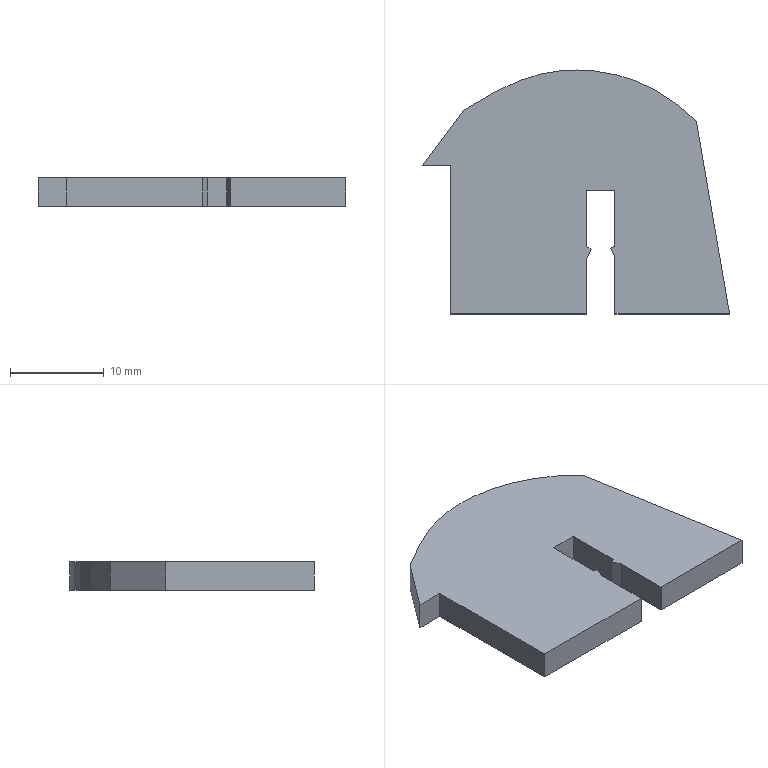Part | SolidWorks | features BaseBody 1 | 1 solid | 19 faces | box 32.694 x 25.985 x 3 mm | volume 1909 mm3 | plane 15 | spline 4
STEP:
#1=CARTESIAN_POINT('',(11.999,19.781,-1.5));
#2=VERTEX_POINT('',#1);
#3=CARTESIAN_POINT('',(15.525,-0.7188,-1.5));
#4=VERTEX_POINT('',#3);
#5=CARTESIAN_POINT('',(11.999,19.781,-1.5));
#6=CARTESIAN_POINT('',(12.867,14.683,-1.5));
#7=CARTESIAN_POINT('',(15.525,-0.7188,-1.5));
#8=B_SPLINE_CURVE_WITH_KNOTS('',2,(#5,#6,#7),.UNSPECIFIED.,.F.,.F.,(3,3),(0.3846,0.4615),.UNSPECIFIED.);
#9=EDGE_CURVE('',#2,#4,#8,.T.);
#10=ORIENTED_EDGE('',*,*,#9,.T.);
#11=CARTESIAN_POINT('',(3.329,-0.7188,-1.5));
#12=VERTEX_POINT('',#11);
#13=CARTESIAN_POINT('',(0.,-0.7188,-1.5));
#14=DIRECTION('',(-1.,0.,0.));
#15=VECTOR('',#14,1000.);
#16=LINE('',#13,#15);
#17=EDGE_CURVE('',#4,#12,#16,.T.);
#18=ORIENTED_EDGE('',*,*,#17,.T.);
#19=CARTESIAN_POINT('',(3.329,5.255,-1.5));
#20=VERTEX_POINT('',#19);
#21=CARTESIAN_POINT('',(3.329,0.,-1.5));
#22=DIRECTION('',(0.,-1.,0.));
#23=VECTOR('',#22,1000.);
#24=LINE('',#21,#23);
#25=EDGE_CURVE('',#20,#12,#24,.T.);
#26=ORIENTED_EDGE('',*,*,#25,.F.);
#27=CARTESIAN_POINT('',(2.879,6.296,-1.5));
#28=VERTEX_POINT('',#27);
#29=CARTESIAN_POINT('',(4.72,2.043,-1.5));
#30=DIRECTION('',(0.3973,-0.9177,0.));
#31=VECTOR('',#30,1000.);
#32=LINE('',#29,#31);
#33=EDGE_CURVE('',#28,#20,#32,.T.);
#34=ORIENTED_EDGE('',*,*,#33,.F.);
#35=CARTESIAN_POINT('',(3.329,6.492,-1.5));
#36=VERTEX_POINT('',#35);
#37=CARTESIAN_POINT('',(-1.842,4.249,-1.5));
#38=DIRECTION('',(-0.9175,-0.3978,0.));
#39=VECTOR('',#38,1000.);
#40=LINE('',#37,#39);
#41=EDGE_CURVE('',#36,#28,#40,.T.);
#42=ORIENTED_EDGE('',*,*,#41,.F.);
#43=CARTESIAN_POINT('',(3.329,12.466,-1.5));
#44=VERTEX_POINT('',#43);
#45=CARTESIAN_POINT('',(3.329,0.,-1.5));
#46=DIRECTION('',(0.,-1.,0.));
#47=VECTOR('',#46,1000.);
#48=LINE('',#45,#47);
#49=EDGE_CURVE('',#44,#36,#48,.T.);
#50=ORIENTED_EDGE('',*,*,#49,.F.);
#51=CARTESIAN_POINT('',(0.3317,12.466,-1.5));
#52=VERTEX_POINT('',#51);
#53=CARTESIAN_POINT('',(0.,12.466,-1.5));
#54=DIRECTION('',(1.,0.,0.));
#55=VECTOR('',#54,1000.);
#56=LINE('',#53,#55);
#57=EDGE_CURVE('',#52,#44,#56,.T.);
#58=ORIENTED_EDGE('',*,*,#57,.F.);
#59=CARTESIAN_POINT('',(0.3337,6.459,-1.5));
#60=VERTEX_POINT('',#59);
#61=CARTESIAN_POINT('',(0.3358,0.0001118,-1.5));
#62=DIRECTION('',(-0.000333,1.,0.));
#63=VECTOR('',#62,1000.);
#64=LINE('',#61,#63);
#65=EDGE_CURVE('',#60,#52,#64,.T.);
#66=ORIENTED_EDGE('',*,*,#65,.F.);
#67=CARTESIAN_POINT('',(0.7826,6.196,-1.5));
#68=VERTEX_POINT('',#67);
#69=CARTESIAN_POINT('',(2.904,4.951,-1.5));
#70=DIRECTION('',(-0.8626,0.5059,0.));
#71=VECTOR('',#70,1000.);
#72=LINE('',#69,#71);
#73=EDGE_CURVE('',#68,#60,#72,.T.);
#74=ORIENTED_EDGE('',*,*,#73,.F.);
#75=CARTESIAN_POINT('',(0.3337,5.236,-1.5));
#76=VERTEX_POINT('',#75);
#77=CARTESIAN_POINT('',(-1.736,0.8121,-1.5));
#78=DIRECTION('',(0.4237,0.9058,0.));
#79=VECTOR('',#78,1000.);
#80=LINE('',#77,#79);
#81=EDGE_CURVE('',#76,#68,#80,.T.);
#82=ORIENTED_EDGE('',*,*,#81,.F.);
#83=CARTESIAN_POINT('',(0.3337,-0.7188,-1.5));
#84=VERTEX_POINT('',#83);
#85=CARTESIAN_POINT('',(0.3337,0.,-1.5));
#86=DIRECTION('',(0.,1.,0.));
#87=VECTOR('',#86,1000.);
#88=LINE('',#85,#87);
#89=EDGE_CURVE('',#84,#76,#88,.T.);
#90=ORIENTED_EDGE('',*,*,#89,.F.);
#91=CARTESIAN_POINT('',(-14.173,-0.7188,-1.5));
#92=VERTEX_POINT('',#91);
#93=CARTESIAN_POINT('',(0.,-0.7188,-1.5));
#94=DIRECTION('',(-1.,0.,0.));
#95=VECTOR('',#94,1000.);
#96=LINE('',#93,#95);
#97=EDGE_CURVE('',#84,#92,#96,.T.);
#98=ORIENTED_EDGE('',*,*,#97,.T.);
#99=CARTESIAN_POINT('',(-14.173,15.089,-1.5));
#100=VERTEX_POINT('',#99);
#101=CARTESIAN_POINT('',(-14.173,0.,-1.5));
#102=DIRECTION('',(0.,1.,0.));
#103=VECTOR('',#102,1000.);
#104=LINE('',#101,#103);
#105=EDGE_CURVE('',#92,#100,#104,.T.);
#106=ORIENTED_EDGE('',*,*,#105,.T.);
#107=CARTESIAN_POINT('',(-17.169,15.089,-1.5));
#108=VERTEX_POINT('',#107);
#109=CARTESIAN_POINT('',(0.,15.089,-1.5));
#110=DIRECTION('',(-1.,0.,0.));
#111=VECTOR('',#110,1000.);
#112=LINE('',#109,#111);
#113=EDGE_CURVE('',#100,#108,#112,.T.);
#114=ORIENTED_EDGE('',*,*,#113,.T.);
#115=CARTESIAN_POINT('',(-12.796,20.955,-1.5));
#116=VERTEX_POINT('',#115);
#117=CARTESIAN_POINT('',(-17.169,15.089,-1.5));
#118=CARTESIAN_POINT('',(-15.712,17.045,-1.5));
#119=CARTESIAN_POINT('',(-14.255,19.001,-1.5));
#120=CARTESIAN_POINT('',(-12.796,20.955,-1.5));
#121=B_SPLINE_CURVE_WITH_KNOTS('',3,(#117,#118,#119,#120),.UNSPECIFIED.,.F.,.F.,(4,4),(0.1538,0.2308),.UNSPECIFIED.);
#122=EDGE_CURVE('',#108,#116,#121,.T.);
#123=ORIENTED_EDGE('',*,*,#122,.T.);
#124=CARTESIAN_POINT('',(1.186,25.157,-1.5));
#125=VERTEX_POINT('',#124);
#126=CARTESIAN_POINT('',(-12.796,20.955,-1.5));
#127=CARTESIAN_POINT('',(-8.856,23.384,-1.5));
#128=CARTESIAN_POINT('',(-4.918,25.815,-1.5));
#129=CARTESIAN_POINT('',(1.186,25.157,-1.5));
#130=B_SPLINE_CURVE_WITH_KNOTS('',3,(#126,#127,#128,#129),.UNSPECIFIED.,.F.,.F.,(4,4),(0.2308,0.3077),.UNSPECIFIED.);
#131=EDGE_CURVE('',#116,#125,#130,.T.);
#132=ORIENTED_EDGE('',*,*,#131,.T.);
#133=CARTESIAN_POINT('',(1.186,25.157,-1.5));
#134=CARTESIAN_POINT('',(5.549,24.686,-1.5));
#135=CARTESIAN_POINT('',(9.134,22.646,-1.5));
#136=CARTESIAN_POINT('',(11.999,19.781,-1.5));
#137=B_SPLINE_CURVE_WITH_KNOTS('',3,(#133,#134,#135,#136),.UNSPECIFIED.,.F.,.F.,(4,4),(0.3077,0.3846),.UNSPECIFIED.);
#138=EDGE_CURVE('',#125,#2,#137,.T.);
#139=ORIENTED_EDGE('',*,*,#138,.T.);
#140=EDGE_LOOP('',(#10,#18,#26,#34,#42,#50,#58,#66,#74,#82,#90,#98,#106,#114,#123,#132,#139));
#141=FACE_OUTER_BOUND('',#140,.T.);
#142=CARTESIAN_POINT('',(0.,0.,-1.5));
#143=DIRECTION('',(0.,0.,1.));
#144=DIRECTION('',(1.,0.,0.));
#145=AXIS2_PLACEMENT_3D('',#142,#143,#144);
#146=PLANE('',#145);
#147=ADVANCED_FACE('',(#141),#146,.F.);
#148=CARTESIAN_POINT('',(11.999,19.781,1.5));
#149=VERTEX_POINT('',#148);
#150=CARTESIAN_POINT('',(15.525,-0.7188,1.5));
#151=VERTEX_POINT('',#150);
#152=CARTESIAN_POINT('',(11.999,19.781,1.5));
#153=CARTESIAN_POINT('',(12.867,14.683,1.5));
#154=CARTESIAN_POINT('',(15.525,-0.7188,1.5));
#155=B_SPLINE_CURVE_WITH_KNOTS('',2,(#152,#153,#154),.UNSPECIFIED.,.F.,.F.,(3,3),(0.3846,0.4615),.UNSPECIFIED.);
#156=EDGE_CURVE('',#149,#151,#155,.T.);
#157=ORIENTED_EDGE('',*,*,#156,.F.);
#158=CARTESIAN_POINT('',(1.186,25.157,1.5));
#159=VERTEX_POINT('',#158);
#160=CARTESIAN_POINT('',(1.186,25.157,1.5));
#161=CARTESIAN_POINT('',(5.549,24.686,1.5));
#162=CARTESIAN_POINT('',(9.134,22.646,1.5));
#163=CARTESIAN_POINT('',(11.999,19.781,1.5));
#164=B_SPLINE_CURVE_WITH_KNOTS('',3,(#160,#161,#162,#163),.UNSPECIFIED.,.F.,.F.,(4,4),(0.3077,0.3846),.UNSPECIFIED.);
#165=EDGE_CURVE('',#159,#149,#164,.T.);
#166=ORIENTED_EDGE('',*,*,#165,.F.);
#167=CARTESIAN_POINT('',(-12.796,20.955,1.5));
#168=VERTEX_POINT('',#167);
#169=CARTESIAN_POINT('',(-12.796,20.955,1.5));
#170=CARTESIAN_POINT('',(-8.856,23.384,1.5));
#171=CARTESIAN_POINT('',(-4.918,25.815,1.5));
#172=CARTESIAN_POINT('',(1.186,25.157,1.5));
#173=B_SPLINE_CURVE_WITH_KNOTS('',3,(#169,#170,#171,#172),.UNSPECIFIED.,.F.,.F.,(4,4),(0.2308,0.3077),.UNSPECIFIED.);
#174=EDGE_CURVE('',#168,#159,#173,.T.);
#175=ORIENTED_EDGE('',*,*,#174,.F.);
#176=CARTESIAN_POINT('',(-17.169,15.089,1.5));
#177=VERTEX_POINT('',#176);
#178=CARTESIAN_POINT('',(-17.169,15.089,1.5));
#179=CARTESIAN_POINT('',(-15.712,17.045,1.5));
#180=CARTESIAN_POINT('',(-14.255,19.001,1.5));
#181=CARTESIAN_POINT('',(-12.796,20.955,1.5));
#182=B_SPLINE_CURVE_WITH_KNOTS('',3,(#178,#179,#180,#181),.UNSPECIFIED.,.F.,.F.,(4,4),(0.1538,0.2308),.UNSPECIFIED.);
#183=EDGE_CURVE('',#177,#168,#182,.T.);
#184=ORIENTED_EDGE('',*,*,#183,.F.);
#185=CARTESIAN_POINT('',(-14.173,15.089,1.5));
#186=VERTEX_POINT('',#185);
#187=CARTESIAN_POINT('',(0.,15.089,1.5));
#188=DIRECTION('',(-1.,0.,0.));
#189=VECTOR('',#188,1000.);
#190=LINE('',#187,#189);
#191=EDGE_CURVE('',#186,#177,#190,.T.);
#192=ORIENTED_EDGE('',*,*,#191,.F.);
#193=CARTESIAN_POINT('',(-14.173,-0.7188,1.5));
#194=VERTEX_POINT('',#193);
#195=CARTESIAN_POINT('',(-14.173,0.,1.5));
#196=DIRECTION('',(0.,1.,0.));
#197=VECTOR('',#196,1000.);
#198=LINE('',#195,#197);
#199=EDGE_CURVE('',#194,#186,#198,.T.);
#200=ORIENTED_EDGE('',*,*,#199,.F.);
#201=CARTESIAN_POINT('',(0.3337,-0.7188,1.5));
#202=VERTEX_POINT('',#201);
#203=CARTESIAN_POINT('',(0.,-0.7188,1.5));
#204=DIRECTION('',(-1.,0.,0.));
#205=VECTOR('',#204,1000.);
#206=LINE('',#203,#205);
#207=EDGE_CURVE('',#202,#194,#206,.T.);
#208=ORIENTED_EDGE('',*,*,#207,.F.);
#209=CARTESIAN_POINT('',(0.3337,5.236,1.5));
#210=VERTEX_POINT('',#209);
#211=CARTESIAN_POINT('',(0.3337,0.,1.5));
#212=DIRECTION('',(0.,1.,0.));
#213=VECTOR('',#212,1000.);
#214=LINE('',#211,#213);
#215=EDGE_CURVE('',#202,#210,#214,.T.);
#216=ORIENTED_EDGE('',*,*,#215,.T.);
#217=CARTESIAN_POINT('',(0.7826,6.196,1.5));
#218=VERTEX_POINT('',#217);
#219=CARTESIAN_POINT('',(-1.736,0.8121,1.5));
#220=DIRECTION('',(0.4237,0.9058,0.));
#221=VECTOR('',#220,1000.);
#222=LINE('',#219,#221);
#223=EDGE_CURVE('',#210,#218,#222,.T.);
#224=ORIENTED_EDGE('',*,*,#223,.T.);
#225=CARTESIAN_POINT('',(0.3337,6.459,1.5));
#226=VERTEX_POINT('',#225);
#227=CARTESIAN_POINT('',(2.904,4.951,1.5));
#228=DIRECTION('',(-0.8626,0.5059,0.));
#229=VECTOR('',#228,1000.);
#230=LINE('',#227,#229);
#231=EDGE_CURVE('',#218,#226,#230,.T.);
#232=ORIENTED_EDGE('',*,*,#231,.T.);
#233=CARTESIAN_POINT('',(0.3317,12.466,1.5));
#234=VERTEX_POINT('',#233);
#235=CARTESIAN_POINT('',(0.3358,0.0001118,1.5));
#236=DIRECTION('',(-0.000333,1.,0.));
#237=VECTOR('',#236,1000.);
#238=LINE('',#235,#237);
#239=EDGE_CURVE('',#226,#234,#238,.T.);
#240=ORIENTED_EDGE('',*,*,#239,.T.);
#241=CARTESIAN_POINT('',(3.329,12.466,1.5));
#242=VERTEX_POINT('',#241);
#243=CARTESIAN_POINT('',(0.,12.466,1.5));
#244=DIRECTION('',(1.,0.,0.));
#245=VECTOR('',#244,1000.);
#246=LINE('',#243,#245);
#247=EDGE_CURVE('',#234,#242,#246,.T.);
#248=ORIENTED_EDGE('',*,*,#247,.T.);
#249=CARTESIAN_POINT('',(3.329,6.492,1.5));
#250=VERTEX_POINT('',#249);
#251=CARTESIAN_POINT('',(3.329,0.,1.5));
#252=DIRECTION('',(0.,-1.,0.));
#253=VECTOR('',#252,1000.);
#254=LINE('',#251,#253);
#255=EDGE_CURVE('',#242,#250,#254,.T.);
#256=ORIENTED_EDGE('',*,*,#255,.T.);
#257=CARTESIAN_POINT('',(2.879,6.296,1.5));
#258=VERTEX_POINT('',#257);
#259=CARTESIAN_POINT('',(-1.842,4.249,1.5));
#260=DIRECTION('',(-0.9175,-0.3978,0.));
#261=VECTOR('',#260,1000.);
#262=LINE('',#259,#261);
#263=EDGE_CURVE('',#250,#258,#262,.T.);
#264=ORIENTED_EDGE('',*,*,#263,.T.);
#265=CARTESIAN_POINT('',(3.329,5.255,1.5));
#266=VERTEX_POINT('',#265);
#267=CARTESIAN_POINT('',(4.72,2.043,1.5));
#268=DIRECTION('',(0.3973,-0.9177,0.));
#269=VECTOR('',#268,1000.);
#270=LINE('',#267,#269);
#271=EDGE_CURVE('',#258,#266,#270,.T.);
#272=ORIENTED_EDGE('',*,*,#271,.T.);
#273=CARTESIAN_POINT('',(3.329,-0.7188,1.5));
#274=VERTEX_POINT('',#273);
#275=CARTESIAN_POINT('',(3.329,0.,1.5));
#276=DIRECTION('',(0.,-1.,0.));
#277=VECTOR('',#276,1000.);
#278=LINE('',#275,#277);
#279=EDGE_CURVE('',#266,#274,#278,.T.);
#280=ORIENTED_EDGE('',*,*,#279,.T.);
#281=CARTESIAN_POINT('',(0.,-0.7188,1.5));
#282=DIRECTION('',(-1.,0.,0.));
#283=VECTOR('',#282,1000.);
#284=LINE('',#281,#283);
#285=EDGE_CURVE('',#151,#274,#284,.T.);
#286=ORIENTED_EDGE('',*,*,#285,.F.);
#287=EDGE_LOOP('',(#157,#166,#175,#184,#192,#200,#208,#216,#224,#232,#240,#248,#256,#264,#272,#280,#286));
#288=FACE_OUTER_BOUND('',#287,.T.);
#289=CARTESIAN_POINT('',(0.,0.,1.5));
#290=DIRECTION('',(0.,0.,1.));
#291=DIRECTION('',(1.,0.,0.));
#292=AXIS2_PLACEMENT_3D('',#289,#290,#291);
#293=PLANE('',#292);
#294=ADVANCED_FACE('',(#288),#293,.T.);
#295=ORIENTED_EDGE('',*,*,#17,.F.);
#296=CARTESIAN_POINT('',(15.525,-0.7188,1.5));
#297=DIRECTION('',(0.,0.,-1.));
#298=VECTOR('',#297,1000.);
#299=LINE('',#296,#298);
#300=EDGE_CURVE('',#151,#4,#299,.T.);
#301=ORIENTED_EDGE('',*,*,#300,.F.);
#302=ORIENTED_EDGE('',*,*,#285,.T.);
#303=CARTESIAN_POINT('',(3.329,-0.7188,1.5));
#304=DIRECTION('',(0.,0.,-1.));
#305=VECTOR('',#304,1000.);
#306=LINE('',#303,#305);
#307=EDGE_CURVE('',#274,#12,#306,.T.);
#308=ORIENTED_EDGE('',*,*,#307,.T.);
#309=EDGE_LOOP('',(#295,#301,#302,#308));
#310=FACE_OUTER_BOUND('',#309,.T.);
#311=CARTESIAN_POINT('',(0.,-0.7188,1.5));
#312=DIRECTION('',(0.,-1.,0.));
#313=DIRECTION('',(0.,0.,-1.));
#314=AXIS2_PLACEMENT_3D('',#311,#312,#313);
#315=PLANE('',#314);
#316=ADVANCED_FACE('',(#310),#315,.T.);
#317=ORIENTED_EDGE('',*,*,#25,.T.);
#318=ORIENTED_EDGE('',*,*,#307,.F.);
#319=ORIENTED_EDGE('',*,*,#279,.F.);
#320=CARTESIAN_POINT('',(3.329,5.255,1.5));
#321=DIRECTION('',(0.,0.,-1.));
#322=VECTOR('',#321,1000.);
#323=LINE('',#320,#322);
#324=EDGE_CURVE('',#266,#20,#323,.T.);
#325=ORIENTED_EDGE('',*,*,#324,.T.);
#326=EDGE_LOOP('',(#317,#318,#319,#325));
#327=FACE_OUTER_BOUND('',#326,.T.);
#328=CARTESIAN_POINT('',(3.329,0.,1.5));
#329=DIRECTION('',(1.,0.,0.));
#330=DIRECTION('',(0.,1.,0.));
#331=AXIS2_PLACEMENT_3D('',#328,#329,#330);
#332=PLANE('',#331);
#333=ADVANCED_FACE('',(#327),#332,.F.);
#334=ORIENTED_EDGE('',*,*,#33,.T.);
#335=ORIENTED_EDGE('',*,*,#324,.F.);
#336=ORIENTED_EDGE('',*,*,#271,.F.);
#337=CARTESIAN_POINT('',(2.879,6.296,1.5));
#338=DIRECTION('',(0.,0.,-1.));
#339=VECTOR('',#338,1000.);
#340=LINE('',#337,#339);
#341=EDGE_CURVE('',#258,#28,#340,.T.);
#342=ORIENTED_EDGE('',*,*,#341,.T.);
#343=EDGE_LOOP('',(#334,#335,#336,#342));
#344=FACE_OUTER_BOUND('',#343,.T.);
#345=CARTESIAN_POINT('',(4.72,2.043,1.5));
#346=DIRECTION('',(0.9177,0.3973,0.));
#347=DIRECTION('',(0.,0.,-1.));
#348=AXIS2_PLACEMENT_3D('',#345,#346,#347);
#349=PLANE('',#348);
#350=ADVANCED_FACE('',(#344),#349,.F.);
#351=ORIENTED_EDGE('',*,*,#41,.T.);
#352=ORIENTED_EDGE('',*,*,#341,.F.);
#353=ORIENTED_EDGE('',*,*,#263,.F.);
#354=CARTESIAN_POINT('',(3.329,6.492,1.5));
#355=DIRECTION('',(0.,0.,-1.));
#356=VECTOR('',#355,1000.);
#357=LINE('',#354,#356);
#358=EDGE_CURVE('',#250,#36,#357,.T.);
#359=ORIENTED_EDGE('',*,*,#358,.T.);
#360=EDGE_LOOP('',(#351,#352,#353,#359));
#361=FACE_OUTER_BOUND('',#360,.T.);
#362=CARTESIAN_POINT('',(-1.842,4.249,1.5));
#363=DIRECTION('',(0.3978,-0.9175,0.));
#364=DIRECTION('',(0.,0.,-1.));
#365=AXIS2_PLACEMENT_3D('',#362,#363,#364);
#366=PLANE('',#365);
#367=ADVANCED_FACE('',(#361),#366,.F.);
#368=ORIENTED_EDGE('',*,*,#49,.T.);
#369=ORIENTED_EDGE('',*,*,#358,.F.);
#370=ORIENTED_EDGE('',*,*,#255,.F.);
#371=CARTESIAN_POINT('',(3.329,12.466,1.5));
#372=DIRECTION('',(0.,0.,-1.));
#373=VECTOR('',#372,1000.);
#374=LINE('',#371,#373);
#375=EDGE_CURVE('',#242,#44,#374,.T.);
#376=ORIENTED_EDGE('',*,*,#375,.T.);
#377=EDGE_LOOP('',(#368,#369,#370,#376));
#378=FACE_OUTER_BOUND('',#377,.T.);
#379=CARTESIAN_POINT('',(3.329,0.,1.5));
#380=DIRECTION('',(1.,0.,0.));
#381=DIRECTION('',(0.,1.,0.));
#382=AXIS2_PLACEMENT_3D('',#379,#380,#381);
#383=PLANE('',#382);
#384=ADVANCED_FACE('',(#378),#383,.F.);
#385=ORIENTED_EDGE('',*,*,#57,.T.);
#386=ORIENTED_EDGE('',*,*,#375,.F.);
#387=ORIENTED_EDGE('',*,*,#247,.F.);
#388=CARTESIAN_POINT('',(0.3317,12.466,1.5));
#389=DIRECTION('',(0.,0.,-1.));
#390=VECTOR('',#389,1000.);
#391=LINE('',#388,#390);
#392=EDGE_CURVE('',#234,#52,#391,.T.);
#393=ORIENTED_EDGE('',*,*,#392,.T.);
#394=EDGE_LOOP('',(#385,#386,#387,#393));
#395=FACE_OUTER_BOUND('',#394,.T.);
#396=CARTESIAN_POINT('',(0.,12.466,1.5));
#397=DIRECTION('',(0.,1.,0.));
#398=DIRECTION('',(1.,0.,0.));
#399=AXIS2_PLACEMENT_3D('',#396,#397,#398);
#400=PLANE('',#399);
#401=ADVANCED_FACE('',(#395),#400,.F.);
#402=ORIENTED_EDGE('',*,*,#65,.T.);
#403=ORIENTED_EDGE('',*,*,#392,.F.);
#404=ORIENTED_EDGE('',*,*,#239,.F.);
#405=CARTESIAN_POINT('',(0.3337,6.459,1.5));
#406=DIRECTION('',(0.,0.,-1.));
#407=VECTOR('',#406,1000.);
#408=LINE('',#405,#407);
#409=EDGE_CURVE('',#226,#60,#408,.T.);
#410=ORIENTED_EDGE('',*,*,#409,.T.);
#411=EDGE_LOOP('',(#402,#403,#404,#410));
#412=FACE_OUTER_BOUND('',#411,.T.);
#413=CARTESIAN_POINT('',(0.3358,0.0001118,1.5));
#414=DIRECTION('',(-1.,-0.000333,0.));
#415=DIRECTION('',(-0.000333,1.,0.));
#416=AXIS2_PLACEMENT_3D('',#413,#414,#415);
#417=PLANE('',#416);
#418=ADVANCED_FACE('',(#412),#417,.F.);
#419=ORIENTED_EDGE('',*,*,#73,.T.);
#420=ORIENTED_EDGE('',*,*,#409,.F.);
#421=ORIENTED_EDGE('',*,*,#231,.F.);
#422=CARTESIAN_POINT('',(0.7826,6.196,1.5));
#423=DIRECTION('',(0.,0.,-1.));
#424=VECTOR('',#423,1000.);
#425=LINE('',#422,#424);
#426=EDGE_CURVE('',#218,#68,#425,.T.);
#427=ORIENTED_EDGE('',*,*,#426,.T.);
#428=EDGE_LOOP('',(#419,#420,#421,#427));
#429=FACE_OUTER_BOUND('',#428,.T.);
#430=CARTESIAN_POINT('',(2.904,4.951,1.5));
#431=DIRECTION('',(-0.5059,-0.8626,0.));
#432=DIRECTION('',(-0.8626,0.5059,0.));
#433=AXIS2_PLACEMENT_3D('',#430,#431,#432);
#434=PLANE('',#433);
#435=ADVANCED_FACE('',(#429),#434,.F.);
#436=ORIENTED_EDGE('',*,*,#81,.T.);
#437=ORIENTED_EDGE('',*,*,#426,.F.);
#438=ORIENTED_EDGE('',*,*,#223,.F.);
#439=CARTESIAN_POINT('',(0.3337,5.236,1.5));
#440=DIRECTION('',(0.,0.,-1.));
#441=VECTOR('',#440,1000.);
#442=LINE('',#439,#441);
#443=EDGE_CURVE('',#210,#76,#442,.T.);
#444=ORIENTED_EDGE('',*,*,#443,.T.);
#445=EDGE_LOOP('',(#436,#437,#438,#444));
#446=FACE_OUTER_BOUND('',#445,.T.);
#447=CARTESIAN_POINT('',(-1.736,0.8121,1.5));
#448=DIRECTION('',(-0.9058,0.4237,0.));
#449=DIRECTION('',(0.,0.,1.));
#450=AXIS2_PLACEMENT_3D('',#447,#448,#449);
#451=PLANE('',#450);
#452=ADVANCED_FACE('',(#446),#451,.F.);
#453=ORIENTED_EDGE('',*,*,#89,.T.);
#454=ORIENTED_EDGE('',*,*,#443,.F.);
#455=ORIENTED_EDGE('',*,*,#215,.F.);
#456=CARTESIAN_POINT('',(0.3337,-0.7188,1.5));
#457=DIRECTION('',(0.,0.,-1.));
#458=VECTOR('',#457,1000.);
#459=LINE('',#456,#458);
#460=EDGE_CURVE('',#202,#84,#459,.T.);
#461=ORIENTED_EDGE('',*,*,#460,.T.);
#462=EDGE_LOOP('',(#453,#454,#455,#461));
#463=FACE_OUTER_BOUND('',#462,.T.);
#464=CARTESIAN_POINT('',(0.3337,0.,1.5));
#465=DIRECTION('',(-1.,0.,0.));
#466=DIRECTION('',(0.,0.,1.));
#467=AXIS2_PLACEMENT_3D('',#464,#465,#466);
#468=PLANE('',#467);
#469=ADVANCED_FACE('',(#463),#468,.F.);
#470=ORIENTED_EDGE('',*,*,#97,.F.);
#471=ORIENTED_EDGE('',*,*,#460,.F.);
#472=ORIENTED_EDGE('',*,*,#207,.T.);
#473=CARTESIAN_POINT('',(-14.173,-0.7188,1.5));
#474=DIRECTION('',(0.,0.,-1.));
#475=VECTOR('',#474,1000.);
#476=LINE('',#473,#475);
#477=EDGE_CURVE('',#194,#92,#476,.T.);
#478=ORIENTED_EDGE('',*,*,#477,.T.);
#479=EDGE_LOOP('',(#470,#471,#472,#478));
#480=FACE_OUTER_BOUND('',#479,.T.);
#481=CARTESIAN_POINT('',(0.,-0.7188,1.5));
#482=DIRECTION('',(0.,-1.,0.));
#483=DIRECTION('',(0.,0.,-1.));
#484=AXIS2_PLACEMENT_3D('',#481,#482,#483);
#485=PLANE('',#484);
#486=ADVANCED_FACE('',(#480),#485,.T.);
#487=ORIENTED_EDGE('',*,*,#105,.F.);
#488=ORIENTED_EDGE('',*,*,#477,.F.);
#489=ORIENTED_EDGE('',*,*,#199,.T.);
#490=CARTESIAN_POINT('',(-14.173,15.089,1.5));
#491=DIRECTION('',(0.,0.,-1.));
#492=VECTOR('',#491,1000.);
#493=LINE('',#490,#492);
#494=EDGE_CURVE('',#186,#100,#493,.T.);
#495=ORIENTED_EDGE('',*,*,#494,.T.);
#496=EDGE_LOOP('',(#487,#488,#489,#495));
#497=FACE_OUTER_BOUND('',#496,.T.);
#498=CARTESIAN_POINT('',(-14.173,0.,1.5));
#499=DIRECTION('',(-1.,0.,0.));
#500=DIRECTION('',(0.,0.,1.));
#501=AXIS2_PLACEMENT_3D('',#498,#499,#500);
#502=PLANE('',#501);
#503=ADVANCED_FACE('',(#497),#502,.T.);
#504=ORIENTED_EDGE('',*,*,#113,.F.);
#505=ORIENTED_EDGE('',*,*,#494,.F.);
#506=ORIENTED_EDGE('',*,*,#191,.T.);
#507=CARTESIAN_POINT('',(-17.169,15.089,1.5));
#508=DIRECTION('',(0.,0.,-1.));
#509=VECTOR('',#508,1000.);
#510=LINE('',#507,#509);
#511=EDGE_CURVE('',#177,#108,#510,.T.);
#512=ORIENTED_EDGE('',*,*,#511,.T.);
#513=EDGE_LOOP('',(#504,#505,#506,#512));
#514=FACE_OUTER_BOUND('',#513,.T.);
#515=CARTESIAN_POINT('',(0.,15.089,1.5));
#516=DIRECTION('',(0.,-1.,0.));
#517=DIRECTION('',(0.,0.,-1.));
#518=AXIS2_PLACEMENT_3D('',#515,#516,#517);
#519=PLANE('',#518);
#520=ADVANCED_FACE('',(#514),#519,.T.);
#521=ORIENTED_EDGE('',*,*,#122,.F.);
#522=ORIENTED_EDGE('',*,*,#511,.F.);
#523=ORIENTED_EDGE('',*,*,#183,.T.);
#524=CARTESIAN_POINT('',(-12.796,20.955,1.5));
#525=DIRECTION('',(0.,0.,-1.));
#526=VECTOR('',#525,1000.);
#527=LINE('',#524,#526);
#528=EDGE_CURVE('',#168,#116,#527,.T.);
#529=ORIENTED_EDGE('',*,*,#528,.T.);
#530=EDGE_LOOP('',(#521,#522,#523,#529));
#531=FACE_OUTER_BOUND('',#530,.T.);
#532=CARTESIAN_POINT('',(-17.169,15.089,1.5));
#533=CARTESIAN_POINT('',(-17.169,15.089,-1.5));
#534=CARTESIAN_POINT('',(-15.712,17.045,1.5));
#535=CARTESIAN_POINT('',(-15.712,17.045,-1.5));
#536=CARTESIAN_POINT('',(-14.255,19.001,1.5));
#537=CARTESIAN_POINT('',(-14.255,19.001,-1.5));
#538=CARTESIAN_POINT('',(-12.796,20.955,1.5));
#539=CARTESIAN_POINT('',(-12.796,20.955,-1.5));
#540=B_SPLINE_SURFACE_WITH_KNOTS('',3,1,((#532,#533),(#534,#535),(#536,#537),(#538,#539)),.UNSPECIFIED.,.F.,.F.,.F.,(4,4),(2,2),(0.1538,0.2308),(0.,1.),.UNSPECIFIED.);
#541=ADVANCED_FACE('',(#531),#540,.T.);
#542=ORIENTED_EDGE('',*,*,#131,.F.);
#543=ORIENTED_EDGE('',*,*,#528,.F.);
#544=ORIENTED_EDGE('',*,*,#174,.T.);
#545=CARTESIAN_POINT('',(1.186,25.157,1.5));
#546=DIRECTION('',(0.,0.,-1.));
#547=VECTOR('',#546,1000.);
#548=LINE('',#545,#547);
#549=EDGE_CURVE('',#159,#125,#548,.T.);
#550=ORIENTED_EDGE('',*,*,#549,.T.);
#551=EDGE_LOOP('',(#542,#543,#544,#550));
#552=FACE_OUTER_BOUND('',#551,.T.);
#553=CARTESIAN_POINT('',(-12.796,20.955,1.5));
#554=CARTESIAN_POINT('',(-12.796,20.955,-1.5));
#555=CARTESIAN_POINT('',(-8.856,23.384,1.5));
#556=CARTESIAN_POINT('',(-8.856,23.384,-1.5));
#557=CARTESIAN_POINT('',(-4.918,25.815,1.5));
#558=CARTESIAN_POINT('',(-4.918,25.815,-1.5));
#559=CARTESIAN_POINT('',(1.186,25.157,1.5));
#560=CARTESIAN_POINT('',(1.186,25.157,-1.5));
#561=B_SPLINE_SURFACE_WITH_KNOTS('',3,1,((#553,#554),(#555,#556),(#557,#558),(#559,#560)),.UNSPECIFIED.,.F.,.F.,.F.,(4,4),(2,2),(0.2308,0.3077),(0.,1.),.UNSPECIFIED.);
#562=ADVANCED_FACE('',(#552),#561,.T.);
#563=ORIENTED_EDGE('',*,*,#138,.F.);
#564=ORIENTED_EDGE('',*,*,#549,.F.);
#565=ORIENTED_EDGE('',*,*,#165,.T.);
#566=CARTESIAN_POINT('',(11.999,19.781,1.5));
#567=DIRECTION('',(0.,0.,-1.));
#568=VECTOR('',#567,1000.);
#569=LINE('',#566,#568);
#570=EDGE_CURVE('',#149,#2,#569,.T.);
#571=ORIENTED_EDGE('',*,*,#570,.T.);
#572=EDGE_LOOP('',(#563,#564,#565,#571));
#573=FACE_OUTER_BOUND('',#572,.T.);
#574=CARTESIAN_POINT('',(1.186,25.157,1.5));
#575=CARTESIAN_POINT('',(1.186,25.157,-1.5));
#576=CARTESIAN_POINT('',(5.549,24.686,1.5));
#577=CARTESIAN_POINT('',(5.549,24.686,-1.5));
#578=CARTESIAN_POINT('',(9.134,22.646,1.5));
#579=CARTESIAN_POINT('',(9.134,22.646,-1.5));
#580=CARTESIAN_POINT('',(11.999,19.781,1.5));
#581=CARTESIAN_POINT('',(11.999,19.781,-1.5));
#582=B_SPLINE_SURFACE_WITH_KNOTS('',3,1,((#574,#575),(#576,#577),(#578,#579),(#580,#581)),.UNSPECIFIED.,.F.,.F.,.F.,(4,4),(2,2),(0.3077,0.3846),(0.,1.),.UNSPECIFIED.);
#583=ADVANCED_FACE('',(#573),#582,.T.);
#584=ORIENTED_EDGE('',*,*,#9,.F.);
#585=ORIENTED_EDGE('',*,*,#570,.F.);
#586=ORIENTED_EDGE('',*,*,#156,.T.);
#587=ORIENTED_EDGE('',*,*,#300,.T.);
#588=EDGE_LOOP('',(#584,#585,#586,#587));
#589=FACE_OUTER_BOUND('',#588,.T.);
#590=CARTESIAN_POINT('',(11.999,19.781,1.5));
#591=CARTESIAN_POINT('',(11.999,19.781,-1.5));
#592=CARTESIAN_POINT('',(12.867,14.683,1.5));
#593=CARTESIAN_POINT('',(12.867,14.683,-1.5));
#594=CARTESIAN_POINT('',(15.525,-0.7188,1.5));
#595=CARTESIAN_POINT('',(15.525,-0.7188,-1.5));
#596=B_SPLINE_SURFACE_WITH_KNOTS('',2,1,((#590,#591),(#592,#593),(#594,#595)),.UNSPECIFIED.,.F.,.F.,.F.,(3,3),(2,2),(0.3846,0.4615),(0.,1.),.UNSPECIFIED.);
#597=ADVANCED_FACE('',(#589),#596,.T.);
#598=CLOSED_SHELL('',(#147,#294,#316,#333,#350,#367,#384,#401,#418,#435,#452,#469,#486,#503,#520,#541,#562,#583,#597));
#599=MANIFOLD_SOLID_BREP('',#598);
#600=CARTESIAN_POINT('',(0.,0.,0.));
#601=DIRECTION('',(0.,0.,1.));
#602=DIRECTION('',(1.,0.,0.));
#603=AXIS2_PLACEMENT_3D('',#600,#601,#602);
#604=(LENGTH_UNIT()NAMED_UNIT(*)SI_UNIT(.MILLI.,.METRE.));
#605=UNCERTAINTY_MEASURE_WITH_UNIT(LENGTH_MEASURE(0.00001),#604,'','');
#606=(NAMED_UNIT(*)PLANE_ANGLE_UNIT()SI_UNIT($,.RADIAN.));
#607=(NAMED_UNIT(*)SI_UNIT($,.STERADIAN.)SOLID_ANGLE_UNIT());
#608=(GEOMETRIC_REPRESENTATION_CONTEXT(3)GLOBAL_UNCERTAINTY_ASSIGNED_CONTEXT((#605))GLOBAL_UNIT_ASSIGNED_CONTEXT((#604,#606,#607))REPRESENTATION_CONTEXT('',''));
#609=ADVANCED_BREP_SHAPE_REPRESENTATION('',(#599,#603),#608);